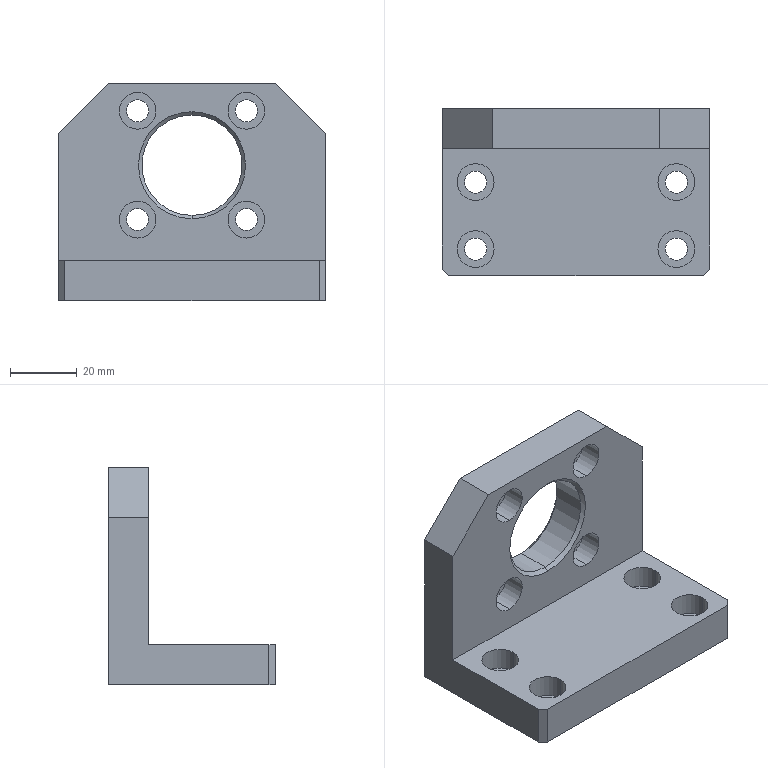Part | SolidWorks | features BaseBody 1 | 1 solid | 58 faces | box 80 x 50 x 65 mm | volume 80960 mm3 | cylinder 34 | plane 20 | cone 4 | commonest cylinder face diameters 6.6 x16 11 x16 30 x2